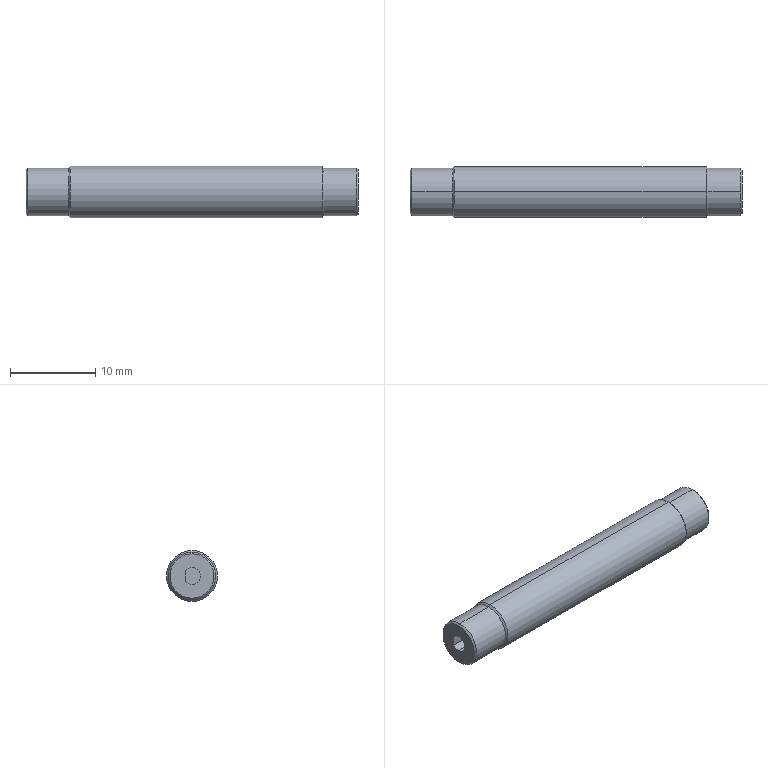Part | SolidWorks | features BaseBody 1 | 1 solid | 21 faces | box 39 x 6 x 6 mm | volume 1057 mm3 | cylinder 9 | cone 8 | plane 4 | commonest cylinder face diameters 5.6 x4 2 x3 6 x2
STEP:
#1=CARTESIAN_POINT('',(34.8,0.,3.));
#2=VERTEX_POINT('',#1);
#3=CARTESIAN_POINT('',(34.8,0.,-3.));
#4=VERTEX_POINT('',#3);
#5=CARTESIAN_POINT('',(34.8,0.,0.));
#6=DIRECTION('',(-1.,0.,0.));
#7=DIRECTION('',(0.,0.,1.));
#8=AXIS2_PLACEMENT_3D('',#5,#6,#7);
#9=CIRCLE('',#8,3.);
#10=EDGE_CURVE('',#2,#4,#9,.T.);
#11=ORIENTED_EDGE('',*,*,#10,.T.);
#12=CARTESIAN_POINT('',(5.2,0.,-3.));
#13=VERTEX_POINT('',#12);
#14=CARTESIAN_POINT('',(0.,0.,-3.));
#15=DIRECTION('',(-1.,0.,0.));
#16=VECTOR('',#15,1000.);
#17=LINE('',#14,#16);
#18=EDGE_CURVE('',#4,#13,#17,.T.);
#19=ORIENTED_EDGE('',*,*,#18,.T.);
#20=CARTESIAN_POINT('',(5.2,0.,3.));
#21=VERTEX_POINT('',#20);
#22=CARTESIAN_POINT('',(5.2,0.,0.));
#23=DIRECTION('',(1.,0.,0.));
#24=DIRECTION('',(0.,0.,1.));
#25=AXIS2_PLACEMENT_3D('',#22,#23,#24);
#26=CIRCLE('',#25,3.);
#27=EDGE_CURVE('',#13,#21,#26,.T.);
#28=ORIENTED_EDGE('',*,*,#27,.T.);
#29=CARTESIAN_POINT('',(0.,0.,3.));
#30=DIRECTION('',(-1.,0.,0.));
#31=VECTOR('',#30,1000.);
#32=LINE('',#29,#31);
#33=EDGE_CURVE('',#2,#21,#32,.T.);
#34=ORIENTED_EDGE('',*,*,#33,.F.);
#35=EDGE_LOOP('',(#11,#19,#28,#34));
#36=FACE_OUTER_BOUND('',#35,.T.);
#37=CARTESIAN_POINT('',(0.,0.,0.));
#38=DIRECTION('',(-1.,0.,0.));
#39=DIRECTION('',(0.,0.,1.));
#40=AXIS2_PLACEMENT_3D('',#37,#38,#39);
#41=CYLINDRICAL_SURFACE('',#40,3.);
#42=ADVANCED_FACE('',(#36),#41,.T.);
#43=CARTESIAN_POINT('',(5.,0.,-2.8));
#44=VERTEX_POINT('',#43);
#45=CARTESIAN_POINT('',(5.,0.,2.8));
#46=VERTEX_POINT('',#45);
#47=CARTESIAN_POINT('',(5.,0.,0.));
#48=DIRECTION('',(1.,0.,0.));
#49=DIRECTION('',(0.,0.,-1.));
#50=AXIS2_PLACEMENT_3D('',#47,#48,#49);
#51=CIRCLE('',#50,2.8);
#52=EDGE_CURVE('',#44,#46,#51,.T.);
#53=ORIENTED_EDGE('',*,*,#52,.T.);
#54=CARTESIAN_POINT('',(5.2,0.,3.));
#55=DIRECTION('',(0.7071,0.,0.7071));
#56=VECTOR('',#55,1000.);
#57=LINE('',#54,#56);
#58=EDGE_CURVE('',#46,#21,#57,.T.);
#59=ORIENTED_EDGE('',*,*,#58,.T.);
#60=ORIENTED_EDGE('',*,*,#27,.F.);
#61=CARTESIAN_POINT('',(5.2,0.,-3.));
#62=DIRECTION('',(0.7071,0.,-0.7071));
#63=VECTOR('',#62,1000.);
#64=LINE('',#61,#63);
#65=EDGE_CURVE('',#44,#13,#64,.T.);
#66=ORIENTED_EDGE('',*,*,#65,.F.);
#67=EDGE_LOOP('',(#53,#59,#60,#66));
#68=FACE_OUTER_BOUND('',#67,.T.);
#69=CARTESIAN_POINT('',(5.2,0.,0.));
#70=DIRECTION('',(1.,0.,0.));
#71=DIRECTION('',(0.,0.,-1.));
#72=AXIS2_PLACEMENT_3D('',#69,#70,#71);
#73=CONICAL_SURFACE('',#72,3.,0.7854);
#74=ADVANCED_FACE('',(#68),#73,.T.);
#75=CARTESIAN_POINT('',(35.,0.,2.8));
#76=VERTEX_POINT('',#75);
#77=CARTESIAN_POINT('',(35.,0.,-2.8));
#78=VERTEX_POINT('',#77);
#79=CARTESIAN_POINT('',(35.,0.,0.));
#80=DIRECTION('',(-1.,0.,0.));
#81=DIRECTION('',(0.,0.,1.));
#82=AXIS2_PLACEMENT_3D('',#79,#80,#81);
#83=CIRCLE('',#82,2.8);
#84=EDGE_CURVE('',#76,#78,#83,.T.);
#85=ORIENTED_EDGE('',*,*,#84,.T.);
#86=CARTESIAN_POINT('',(34.8,0.,-3.));
#87=DIRECTION('',(-0.7071,0.,-0.7071));
#88=VECTOR('',#87,1000.);
#89=LINE('',#86,#88);
#90=EDGE_CURVE('',#78,#4,#89,.T.);
#91=ORIENTED_EDGE('',*,*,#90,.T.);
#92=ORIENTED_EDGE('',*,*,#10,.F.);
#93=CARTESIAN_POINT('',(34.8,0.,3.));
#94=DIRECTION('',(-0.7071,0.,0.7071));
#95=VECTOR('',#94,1000.);
#96=LINE('',#93,#95);
#97=EDGE_CURVE('',#76,#2,#96,.T.);
#98=ORIENTED_EDGE('',*,*,#97,.F.);
#99=EDGE_LOOP('',(#85,#91,#92,#98));
#100=FACE_OUTER_BOUND('',#99,.T.);
#101=CARTESIAN_POINT('',(34.8,0.,0.));
#102=DIRECTION('',(-1.,0.,0.));
#103=DIRECTION('',(0.,0.,1.));
#104=AXIS2_PLACEMENT_3D('',#101,#102,#103);
#105=CONICAL_SURFACE('',#104,3.,0.7854);
#106=ADVANCED_FACE('',(#100),#105,.T.);
#107=ORIENTED_EDGE('',*,*,#52,.F.);
#108=CARTESIAN_POINT('',(0.2,0.,-2.8));
#109=VERTEX_POINT('',#108);
#110=CARTESIAN_POINT('',(0.,0.,-2.8));
#111=DIRECTION('',(-1.,0.,0.));
#112=VECTOR('',#111,1000.);
#113=LINE('',#110,#112);
#114=EDGE_CURVE('',#44,#109,#113,.T.);
#115=ORIENTED_EDGE('',*,*,#114,.T.);
#116=CARTESIAN_POINT('',(0.2,0.,2.8));
#117=VERTEX_POINT('',#116);
#118=CARTESIAN_POINT('',(0.2,0.,0.));
#119=DIRECTION('',(1.,0.,0.));
#120=DIRECTION('',(0.,0.,1.));
#121=AXIS2_PLACEMENT_3D('',#118,#119,#120);
#122=CIRCLE('',#121,2.8);
#123=EDGE_CURVE('',#109,#117,#122,.T.);
#124=ORIENTED_EDGE('',*,*,#123,.T.);
#125=CARTESIAN_POINT('',(0.,0.,2.8));
#126=DIRECTION('',(-1.,0.,0.));
#127=VECTOR('',#126,1000.);
#128=LINE('',#125,#127);
#129=EDGE_CURVE('',#46,#117,#128,.T.);
#130=ORIENTED_EDGE('',*,*,#129,.F.);
#131=EDGE_LOOP('',(#107,#115,#124,#130));
#132=FACE_OUTER_BOUND('',#131,.T.);
#133=CARTESIAN_POINT('',(0.,0.,0.));
#134=DIRECTION('',(-1.,0.,0.));
#135=DIRECTION('',(0.,0.,1.));
#136=AXIS2_PLACEMENT_3D('',#133,#134,#135);
#137=CYLINDRICAL_SURFACE('',#136,2.8);
#138=ADVANCED_FACE('',(#132),#137,.T.);
#139=CARTESIAN_POINT('',(38.8,0.,2.8));
#140=VERTEX_POINT('',#139);
#141=CARTESIAN_POINT('',(38.8,0.,-2.8));
#142=VERTEX_POINT('',#141);
#143=CARTESIAN_POINT('',(38.8,0.,0.));
#144=DIRECTION('',(-1.,0.,0.));
#145=DIRECTION('',(0.,0.,1.));
#146=AXIS2_PLACEMENT_3D('',#143,#144,#145);
#147=CIRCLE('',#146,2.8);
#148=EDGE_CURVE('',#140,#142,#147,.T.);
#149=ORIENTED_EDGE('',*,*,#148,.T.);
#150=CARTESIAN_POINT('',(0.,0.,-2.8));
#151=DIRECTION('',(-1.,0.,0.));
#152=VECTOR('',#151,1000.);
#153=LINE('',#150,#152);
#154=EDGE_CURVE('',#142,#78,#153,.T.);
#155=ORIENTED_EDGE('',*,*,#154,.T.);
#156=ORIENTED_EDGE('',*,*,#84,.F.);
#157=CARTESIAN_POINT('',(0.,0.,2.8));
#158=DIRECTION('',(-1.,0.,0.));
#159=VECTOR('',#158,1000.);
#160=LINE('',#157,#159);
#161=EDGE_CURVE('',#140,#76,#160,.T.);
#162=ORIENTED_EDGE('',*,*,#161,.F.);
#163=EDGE_LOOP('',(#149,#155,#156,#162));
#164=FACE_OUTER_BOUND('',#163,.T.);
#165=CARTESIAN_POINT('',(0.,0.,0.));
#166=DIRECTION('',(-1.,0.,0.));
#167=DIRECTION('',(0.,0.,1.));
#168=AXIS2_PLACEMENT_3D('',#165,#166,#167);
#169=CYLINDRICAL_SURFACE('',#168,2.8);
#170=ADVANCED_FACE('',(#164),#169,.T.);
#171=CARTESIAN_POINT('',(0.,0.,-2.6));
#172=VERTEX_POINT('',#171);
#173=CARTESIAN_POINT('',(0.,0.,2.6));
#174=VERTEX_POINT('',#173);
#175=CARTESIAN_POINT('',(0.,0.,0.));
#176=DIRECTION('',(1.,0.,0.));
#177=DIRECTION('',(0.,0.,-1.));
#178=AXIS2_PLACEMENT_3D('',#175,#176,#177);
#179=CIRCLE('',#178,2.6);
#180=EDGE_CURVE('',#172,#174,#179,.T.);
#181=ORIENTED_EDGE('',*,*,#180,.T.);
#182=CARTESIAN_POINT('',(0.2,0.,2.8));
#183=DIRECTION('',(0.7071,0.,0.7071));
#184=VECTOR('',#183,1000.);
#185=LINE('',#182,#184);
#186=EDGE_CURVE('',#174,#117,#185,.T.);
#187=ORIENTED_EDGE('',*,*,#186,.T.);
#188=ORIENTED_EDGE('',*,*,#123,.F.);
#189=CARTESIAN_POINT('',(0.2,0.,-2.8));
#190=DIRECTION('',(0.7071,0.,-0.7071));
#191=VECTOR('',#190,1000.);
#192=LINE('',#189,#191);
#193=EDGE_CURVE('',#172,#109,#192,.T.);
#194=ORIENTED_EDGE('',*,*,#193,.F.);
#195=EDGE_LOOP('',(#181,#187,#188,#194));
#196=FACE_OUTER_BOUND('',#195,.T.);
#197=CARTESIAN_POINT('',(0.2,0.,0.));
#198=DIRECTION('',(1.,0.,0.));
#199=DIRECTION('',(0.,0.,-1.));
#200=AXIS2_PLACEMENT_3D('',#197,#198,#199);
#201=CONICAL_SURFACE('',#200,2.8,0.7854);
#202=ADVANCED_FACE('',(#196),#201,.T.);
#203=CARTESIAN_POINT('',(39.,0.,2.6));
#204=VERTEX_POINT('',#203);
#205=CARTESIAN_POINT('',(39.,0.,-2.6));
#206=VERTEX_POINT('',#205);
#207=CARTESIAN_POINT('',(39.,0.,0.));
#208=DIRECTION('',(-1.,0.,0.));
#209=DIRECTION('',(0.,0.,1.));
#210=AXIS2_PLACEMENT_3D('',#207,#208,#209);
#211=CIRCLE('',#210,2.6);
#212=EDGE_CURVE('',#204,#206,#211,.T.);
#213=ORIENTED_EDGE('',*,*,#212,.T.);
#214=CARTESIAN_POINT('',(38.8,0.,-2.8));
#215=DIRECTION('',(-0.7071,0.,-0.7071));
#216=VECTOR('',#215,1000.);
#217=LINE('',#214,#216);
#218=EDGE_CURVE('',#206,#142,#217,.T.);
#219=ORIENTED_EDGE('',*,*,#218,.T.);
#220=ORIENTED_EDGE('',*,*,#148,.F.);
#221=CARTESIAN_POINT('',(38.8,0.,2.8));
#222=DIRECTION('',(-0.7071,0.,0.7071));
#223=VECTOR('',#222,1000.);
#224=LINE('',#221,#223);
#225=EDGE_CURVE('',#204,#140,#224,.T.);
#226=ORIENTED_EDGE('',*,*,#225,.F.);
#227=EDGE_LOOP('',(#213,#219,#220,#226));
#228=FACE_OUTER_BOUND('',#227,.T.);
#229=CARTESIAN_POINT('',(38.8,0.,0.));
#230=DIRECTION('',(-1.,0.,0.));
#231=DIRECTION('',(0.,0.,1.));
#232=AXIS2_PLACEMENT_3D('',#229,#230,#231);
#233=CONICAL_SURFACE('',#232,2.8,0.7854);
#234=ADVANCED_FACE('',(#228),#233,.T.);
#235=CARTESIAN_POINT('',(4.,0.,-1.));
#236=VERTEX_POINT('',#235);
#237=CARTESIAN_POINT('',(4.,0.,1.));
#238=VERTEX_POINT('',#237);
#239=CARTESIAN_POINT('',(4.,0.,0.));
#240=DIRECTION('',(-1.,0.,0.));
#241=DIRECTION('',(0.,0.,1.));
#242=AXIS2_PLACEMENT_3D('',#239,#240,#241);
#243=CIRCLE('',#242,1.);
#244=EDGE_CURVE('',#236,#238,#243,.T.);
#245=ORIENTED_EDGE('',*,*,#244,.F.);
#246=CARTESIAN_POINT('',(0.,0.,-1.));
#247=VERTEX_POINT('',#246);
#248=CARTESIAN_POINT('',(4.,0.,-1.));
#249=DIRECTION('',(-1.,0.,0.));
#250=VECTOR('',#249,1000.);
#251=LINE('',#248,#250);
#252=EDGE_CURVE('',#236,#247,#251,.T.);
#253=ORIENTED_EDGE('',*,*,#252,.T.);
#254=CARTESIAN_POINT('',(0.,0.,1.));
#255=VERTEX_POINT('',#254);
#256=CARTESIAN_POINT('',(0.,0.,0.));
#257=DIRECTION('',(-1.,0.,0.));
#258=DIRECTION('',(0.,0.,1.));
#259=AXIS2_PLACEMENT_3D('',#256,#257,#258);
#260=CIRCLE('',#259,1.);
#261=EDGE_CURVE('',#247,#255,#260,.T.);
#262=ORIENTED_EDGE('',*,*,#261,.T.);
#263=CARTESIAN_POINT('',(4.,0.,1.));
#264=DIRECTION('',(-1.,0.,0.));
#265=VECTOR('',#264,1000.);
#266=LINE('',#263,#265);
#267=EDGE_CURVE('',#238,#255,#266,.T.);
#268=ORIENTED_EDGE('',*,*,#267,.F.);
#269=EDGE_LOOP('',(#245,#253,#262,#268));
#270=FACE_OUTER_BOUND('',#269,.T.);
#271=CARTESIAN_POINT('',(4.,0.,0.));
#272=DIRECTION('',(-1.,0.,0.));
#273=DIRECTION('',(0.,0.,1.));
#274=AXIS2_PLACEMENT_3D('',#271,#272,#273);
#275=CYLINDRICAL_SURFACE('',#274,1.);
#276=ADVANCED_FACE('',(#270),#275,.F.);
#277=CARTESIAN_POINT('',(4.,0.8,0.6));
#278=VERTEX_POINT('',#277);
#279=CARTESIAN_POINT('',(4.,0.,0.));
#280=DIRECTION('',(-1.,0.,0.));
#281=DIRECTION('',(0.,0.,1.));
#282=AXIS2_PLACEMENT_3D('',#279,#280,#281);
#283=CIRCLE('',#282,1.);
#284=EDGE_CURVE('',#238,#278,#283,.T.);
#285=ORIENTED_EDGE('',*,*,#284,.F.);
#286=ORIENTED_EDGE('',*,*,#267,.T.);
#287=CARTESIAN_POINT('',(0.,0.8,0.6));
#288=VERTEX_POINT('',#287);
#289=CARTESIAN_POINT('',(0.,0.,0.));
#290=DIRECTION('',(-1.,0.,0.));
#291=DIRECTION('',(0.,0.,1.));
#292=AXIS2_PLACEMENT_3D('',#289,#290,#291);
#293=CIRCLE('',#292,1.);
#294=EDGE_CURVE('',#255,#288,#293,.T.);
#295=ORIENTED_EDGE('',*,*,#294,.T.);
#296=CARTESIAN_POINT('',(4.,0.8,0.6));
#297=DIRECTION('',(-1.,0.,0.));
#298=VECTOR('',#297,1000.);
#299=LINE('',#296,#298);
#300=EDGE_CURVE('',#278,#288,#299,.T.);
#301=ORIENTED_EDGE('',*,*,#300,.F.);
#302=EDGE_LOOP('',(#285,#286,#295,#301));
#303=FACE_OUTER_BOUND('',#302,.T.);
#304=CARTESIAN_POINT('',(4.,0.,0.));
#305=DIRECTION('',(-1.,0.,0.));
#306=DIRECTION('',(0.,0.,1.));
#307=AXIS2_PLACEMENT_3D('',#304,#305,#306);
#308=CYLINDRICAL_SURFACE('',#307,1.);
#309=ADVANCED_FACE('',(#303),#308,.F.);
#310=ORIENTED_EDGE('',*,*,#18,.F.);
#311=CARTESIAN_POINT('',(34.8,0.,0.));
#312=DIRECTION('',(-1.,0.,0.));
#313=DIRECTION('',(0.,0.,1.));
#314=AXIS2_PLACEMENT_3D('',#311,#312,#313);
#315=CIRCLE('',#314,3.);
#316=EDGE_CURVE('',#4,#2,#315,.T.);
#317=ORIENTED_EDGE('',*,*,#316,.T.);
#318=ORIENTED_EDGE('',*,*,#33,.T.);
#319=CARTESIAN_POINT('',(5.2,0.,0.));
#320=DIRECTION('',(1.,0.,0.));
#321=DIRECTION('',(0.,0.,1.));
#322=AXIS2_PLACEMENT_3D('',#319,#320,#321);
#323=CIRCLE('',#322,3.);
#324=EDGE_CURVE('',#21,#13,#323,.T.);
#325=ORIENTED_EDGE('',*,*,#324,.T.);
#326=EDGE_LOOP('',(#310,#317,#318,#325));
#327=FACE_OUTER_BOUND('',#326,.T.);
#328=CARTESIAN_POINT('',(0.,0.,0.));
#329=DIRECTION('',(-1.,0.,0.));
#330=DIRECTION('',(0.,0.,1.));
#331=AXIS2_PLACEMENT_3D('',#328,#329,#330);
#332=CYLINDRICAL_SURFACE('',#331,3.);
#333=ADVANCED_FACE('',(#327),#332,.T.);
#334=ORIENTED_EDGE('',*,*,#58,.F.);
#335=CARTESIAN_POINT('',(5.,0.,0.));
#336=DIRECTION('',(1.,0.,0.));
#337=DIRECTION('',(0.,0.,-1.));
#338=AXIS2_PLACEMENT_3D('',#335,#336,#337);
#339=CIRCLE('',#338,2.8);
#340=EDGE_CURVE('',#46,#44,#339,.T.);
#341=ORIENTED_EDGE('',*,*,#340,.T.);
#342=ORIENTED_EDGE('',*,*,#65,.T.);
#343=ORIENTED_EDGE('',*,*,#324,.F.);
#344=EDGE_LOOP('',(#334,#341,#342,#343));
#345=FACE_OUTER_BOUND('',#344,.T.);
#346=CARTESIAN_POINT('',(5.2,0.,0.));
#347=DIRECTION('',(1.,0.,0.));
#348=DIRECTION('',(0.,0.,-1.));
#349=AXIS2_PLACEMENT_3D('',#346,#347,#348);
#350=CONICAL_SURFACE('',#349,3.,0.7854);
#351=ADVANCED_FACE('',(#345),#350,.T.);
#352=ORIENTED_EDGE('',*,*,#90,.F.);
#353=CARTESIAN_POINT('',(35.,0.,0.));
#354=DIRECTION('',(-1.,0.,0.));
#355=DIRECTION('',(0.,0.,1.));
#356=AXIS2_PLACEMENT_3D('',#353,#354,#355);
#357=CIRCLE('',#356,2.8);
#358=EDGE_CURVE('',#78,#76,#357,.T.);
#359=ORIENTED_EDGE('',*,*,#358,.T.);
#360=ORIENTED_EDGE('',*,*,#97,.T.);
#361=ORIENTED_EDGE('',*,*,#316,.F.);
#362=EDGE_LOOP('',(#352,#359,#360,#361));
#363=FACE_OUTER_BOUND('',#362,.T.);
#364=CARTESIAN_POINT('',(34.8,0.,0.));
#365=DIRECTION('',(-1.,0.,0.));
#366=DIRECTION('',(0.,0.,1.));
#367=AXIS2_PLACEMENT_3D('',#364,#365,#366);
#368=CONICAL_SURFACE('',#367,3.,0.7854);
#369=ADVANCED_FACE('',(#363),#368,.T.);
#370=ORIENTED_EDGE('',*,*,#114,.F.);
#371=ORIENTED_EDGE('',*,*,#340,.F.);
#372=ORIENTED_EDGE('',*,*,#129,.T.);
#373=CARTESIAN_POINT('',(0.2,0.,0.));
#374=DIRECTION('',(1.,0.,0.));
#375=DIRECTION('',(0.,0.,1.));
#376=AXIS2_PLACEMENT_3D('',#373,#374,#375);
#377=CIRCLE('',#376,2.8);
#378=EDGE_CURVE('',#117,#109,#377,.T.);
#379=ORIENTED_EDGE('',*,*,#378,.T.);
#380=EDGE_LOOP('',(#370,#371,#372,#379));
#381=FACE_OUTER_BOUND('',#380,.T.);
#382=CARTESIAN_POINT('',(0.,0.,0.));
#383=DIRECTION('',(-1.,0.,0.));
#384=DIRECTION('',(0.,0.,1.));
#385=AXIS2_PLACEMENT_3D('',#382,#383,#384);
#386=CYLINDRICAL_SURFACE('',#385,2.8);
#387=ADVANCED_FACE('',(#381),#386,.T.);
#388=ORIENTED_EDGE('',*,*,#154,.F.);
#389=CARTESIAN_POINT('',(38.8,0.,0.));
#390=DIRECTION('',(-1.,0.,0.));
#391=DIRECTION('',(0.,0.,1.));
#392=AXIS2_PLACEMENT_3D('',#389,#390,#391);
#393=CIRCLE('',#392,2.8);
#394=EDGE_CURVE('',#142,#140,#393,.T.);
#395=ORIENTED_EDGE('',*,*,#394,.T.);
#396=ORIENTED_EDGE('',*,*,#161,.T.);
#397=ORIENTED_EDGE('',*,*,#358,.F.);
#398=EDGE_LOOP('',(#388,#395,#396,#397));
#399=FACE_OUTER_BOUND('',#398,.T.);
#400=CARTESIAN_POINT('',(0.,0.,0.));
#401=DIRECTION('',(-1.,0.,0.));
#402=DIRECTION('',(0.,0.,1.));
#403=AXIS2_PLACEMENT_3D('',#400,#401,#402);
#404=CYLINDRICAL_SURFACE('',#403,2.8);
#405=ADVANCED_FACE('',(#399),#404,.T.);
#406=ORIENTED_EDGE('',*,*,#186,.F.);
#407=CARTESIAN_POINT('',(0.,0.,0.));
#408=DIRECTION('',(1.,0.,0.));
#409=DIRECTION('',(0.,0.,-1.));
#410=AXIS2_PLACEMENT_3D('',#407,#408,#409);
#411=CIRCLE('',#410,2.6);
#412=EDGE_CURVE('',#174,#172,#411,.T.);
#413=ORIENTED_EDGE('',*,*,#412,.T.);
#414=ORIENTED_EDGE('',*,*,#193,.T.);
#415=ORIENTED_EDGE('',*,*,#378,.F.);
#416=EDGE_LOOP('',(#406,#413,#414,#415));
#417=FACE_OUTER_BOUND('',#416,.T.);
#418=CARTESIAN_POINT('',(0.2,0.,0.));
#419=DIRECTION('',(1.,0.,0.));
#420=DIRECTION('',(0.,0.,-1.));
#421=AXIS2_PLACEMENT_3D('',#418,#419,#420);
#422=CONICAL_SURFACE('',#421,2.8,0.7854);
#423=ADVANCED_FACE('',(#417),#422,.T.);
#424=ORIENTED_EDGE('',*,*,#218,.F.);
#425=CARTESIAN_POINT('',(39.,0.,0.));
#426=DIRECTION('',(-1.,0.,0.));
#427=DIRECTION('',(0.,0.,1.));
#428=AXIS2_PLACEMENT_3D('',#425,#426,#427);
#429=CIRCLE('',#428,2.6);
#430=EDGE_CURVE('',#206,#204,#429,.T.);
#431=ORIENTED_EDGE('',*,*,#430,.T.);
#432=ORIENTED_EDGE('',*,*,#225,.T.);
#433=ORIENTED_EDGE('',*,*,#394,.F.);
#434=EDGE_LOOP('',(#424,#431,#432,#433));
#435=FACE_OUTER_BOUND('',#434,.T.);
#436=CARTESIAN_POINT('',(38.8,0.,0.));
#437=DIRECTION('',(-1.,0.,0.));
#438=DIRECTION('',(0.,0.,1.));
#439=AXIS2_PLACEMENT_3D('',#436,#437,#438);
#440=CONICAL_SURFACE('',#439,2.8,0.7854);
#441=ADVANCED_FACE('',(#435),#440,.T.);
#442=CARTESIAN_POINT('',(0.,0.8,-0.6));
#443=VERTEX_POINT('',#442);
#444=CARTESIAN_POINT('',(0.,0.8,0.));
#445=DIRECTION('',(0.,0.,-1.));
#446=VECTOR('',#445,1000.);
#447=LINE('',#444,#446);
#448=EDGE_CURVE('',#288,#443,#447,.T.);
#449=ORIENTED_EDGE('',*,*,#448,.F.);
#450=ORIENTED_EDGE('',*,*,#294,.F.);
#451=ORIENTED_EDGE('',*,*,#261,.F.);
#452=CARTESIAN_POINT('',(0.,0.,0.));
#453=DIRECTION('',(-1.,0.,0.));
#454=DIRECTION('',(0.,0.,1.));
#455=AXIS2_PLACEMENT_3D('',#452,#453,#454);
#456=CIRCLE('',#455,1.);
#457=EDGE_CURVE('',#443,#247,#456,.T.);
#458=ORIENTED_EDGE('',*,*,#457,.F.);
#459=EDGE_LOOP('',(#449,#450,#451,#458));
#460=FACE_BOUND('',#459,.T.);
#461=ORIENTED_EDGE('',*,*,#180,.F.);
#462=ORIENTED_EDGE('',*,*,#412,.F.);
#463=EDGE_LOOP('',(#461,#462));
#464=FACE_OUTER_BOUND('',#463,.T.);
#465=CARTESIAN_POINT('',(0.,2.8,0.));
#466=DIRECTION('',(1.,0.,0.));
#467=DIRECTION('',(0.,0.,-1.));
#468=AXIS2_PLACEMENT_3D('',#465,#466,#467);
#469=PLANE('',#468);
#470=ADVANCED_FACE('',(#460,#464),#469,.F.);
#471=ORIENTED_EDGE('',*,*,#212,.F.);
#472=ORIENTED_EDGE('',*,*,#430,.F.);
#473=EDGE_LOOP('',(#471,#472));
#474=FACE_OUTER_BOUND('',#473,.T.);
#475=CARTESIAN_POINT('',(39.,2.8,0.));
#476=DIRECTION('',(-1.,0.,0.));
#477=DIRECTION('',(0.,0.,1.));
#478=AXIS2_PLACEMENT_3D('',#475,#476,#477);
#479=PLANE('',#478);
#480=ADVANCED_FACE('',(#474),#479,.F.);
#481=ORIENTED_EDGE('',*,*,#252,.F.);
#482=CARTESIAN_POINT('',(4.,0.8,-0.6));
#483=VERTEX_POINT('',#482);
#484=CARTESIAN_POINT('',(4.,0.,0.));
#485=DIRECTION('',(-1.,0.,0.));
#486=DIRECTION('',(0.,0.,1.));
#487=AXIS2_PLACEMENT_3D('',#484,#485,#486);
#488=CIRCLE('',#487,1.);
#489=EDGE_CURVE('',#483,#236,#488,.T.);
#490=ORIENTED_EDGE('',*,*,#489,.F.);
#491=CARTESIAN_POINT('',(4.,0.8,-0.6));
#492=DIRECTION('',(1.,0.,0.));
#493=VECTOR('',#492,1000.);
#494=LINE('',#491,#493);
#495=EDGE_CURVE('',#443,#483,#494,.T.);
#496=ORIENTED_EDGE('',*,*,#495,.F.);
#497=ORIENTED_EDGE('',*,*,#457,.T.);
#498=EDGE_LOOP('',(#481,#490,#496,#497));
#499=FACE_OUTER_BOUND('',#498,.T.);
#500=CARTESIAN_POINT('',(4.,0.,0.));
#501=DIRECTION('',(-1.,0.,0.));
#502=DIRECTION('',(0.,0.,1.));
#503=AXIS2_PLACEMENT_3D('',#500,#501,#502);
#504=CYLINDRICAL_SURFACE('',#503,1.);
#505=ADVANCED_FACE('',(#499),#504,.F.);
#506=ORIENTED_EDGE('',*,*,#489,.T.);
#507=ORIENTED_EDGE('',*,*,#244,.T.);
#508=ORIENTED_EDGE('',*,*,#284,.T.);
#509=CARTESIAN_POINT('',(4.,0.8,0.));
#510=DIRECTION('',(0.,0.,1.));
#511=VECTOR('',#510,1000.);
#512=LINE('',#509,#511);
#513=EDGE_CURVE('',#483,#278,#512,.T.);
#514=ORIENTED_EDGE('',*,*,#513,.F.);
#515=EDGE_LOOP('',(#506,#507,#508,#514));
#516=FACE_OUTER_BOUND('',#515,.T.);
#517=CARTESIAN_POINT('',(4.,0.,0.));
#518=DIRECTION('',(-1.,0.,0.));
#519=DIRECTION('',(0.,0.,1.));
#520=AXIS2_PLACEMENT_3D('',#517,#518,#519);
#521=PLANE('',#520);
#522=ADVANCED_FACE('',(#516),#521,.T.);
#523=ORIENTED_EDGE('',*,*,#513,.T.);
#524=ORIENTED_EDGE('',*,*,#300,.T.);
#525=ORIENTED_EDGE('',*,*,#448,.T.);
#526=ORIENTED_EDGE('',*,*,#495,.T.);
#527=EDGE_LOOP('',(#523,#524,#525,#526));
#528=FACE_OUTER_BOUND('',#527,.T.);
#529=CARTESIAN_POINT('',(4.,0.8,0.));
#530=DIRECTION('',(0.,-1.,0.));
#531=DIRECTION('',(0.,0.,-1.));
#532=AXIS2_PLACEMENT_3D('',#529,#530,#531);
#533=PLANE('',#532);
#534=ADVANCED_FACE('',(#528),#533,.T.);
#535=CLOSED_SHELL('',(#42,#74,#106,#138,#170,#202,#234,#276,#309,#333,#351,#369,#387,#405,#423,#441,#470,#480,#505,#522,#534));
#536=MANIFOLD_SOLID_BREP('',#535);
#537=CARTESIAN_POINT('',(0.,0.,0.));
#538=DIRECTION('',(0.,0.,1.));
#539=DIRECTION('',(1.,0.,0.));
#540=AXIS2_PLACEMENT_3D('',#537,#538,#539);
#541=(LENGTH_UNIT()NAMED_UNIT(*)SI_UNIT(.MILLI.,.METRE.));
#542=UNCERTAINTY_MEASURE_WITH_UNIT(LENGTH_MEASURE(0.00001),#541,'','');
#543=(NAMED_UNIT(*)PLANE_ANGLE_UNIT()SI_UNIT($,.RADIAN.));
#544=(NAMED_UNIT(*)SI_UNIT($,.STERADIAN.)SOLID_ANGLE_UNIT());
#545=(GEOMETRIC_REPRESENTATION_CONTEXT(3)GLOBAL_UNCERTAINTY_ASSIGNED_CONTEXT((#542))GLOBAL_UNIT_ASSIGNED_CONTEXT((#541,#543,#544))REPRESENTATION_CONTEXT('',''));
#546=ADVANCED_BREP_SHAPE_REPRESENTATION('',(#536,#540),#545);